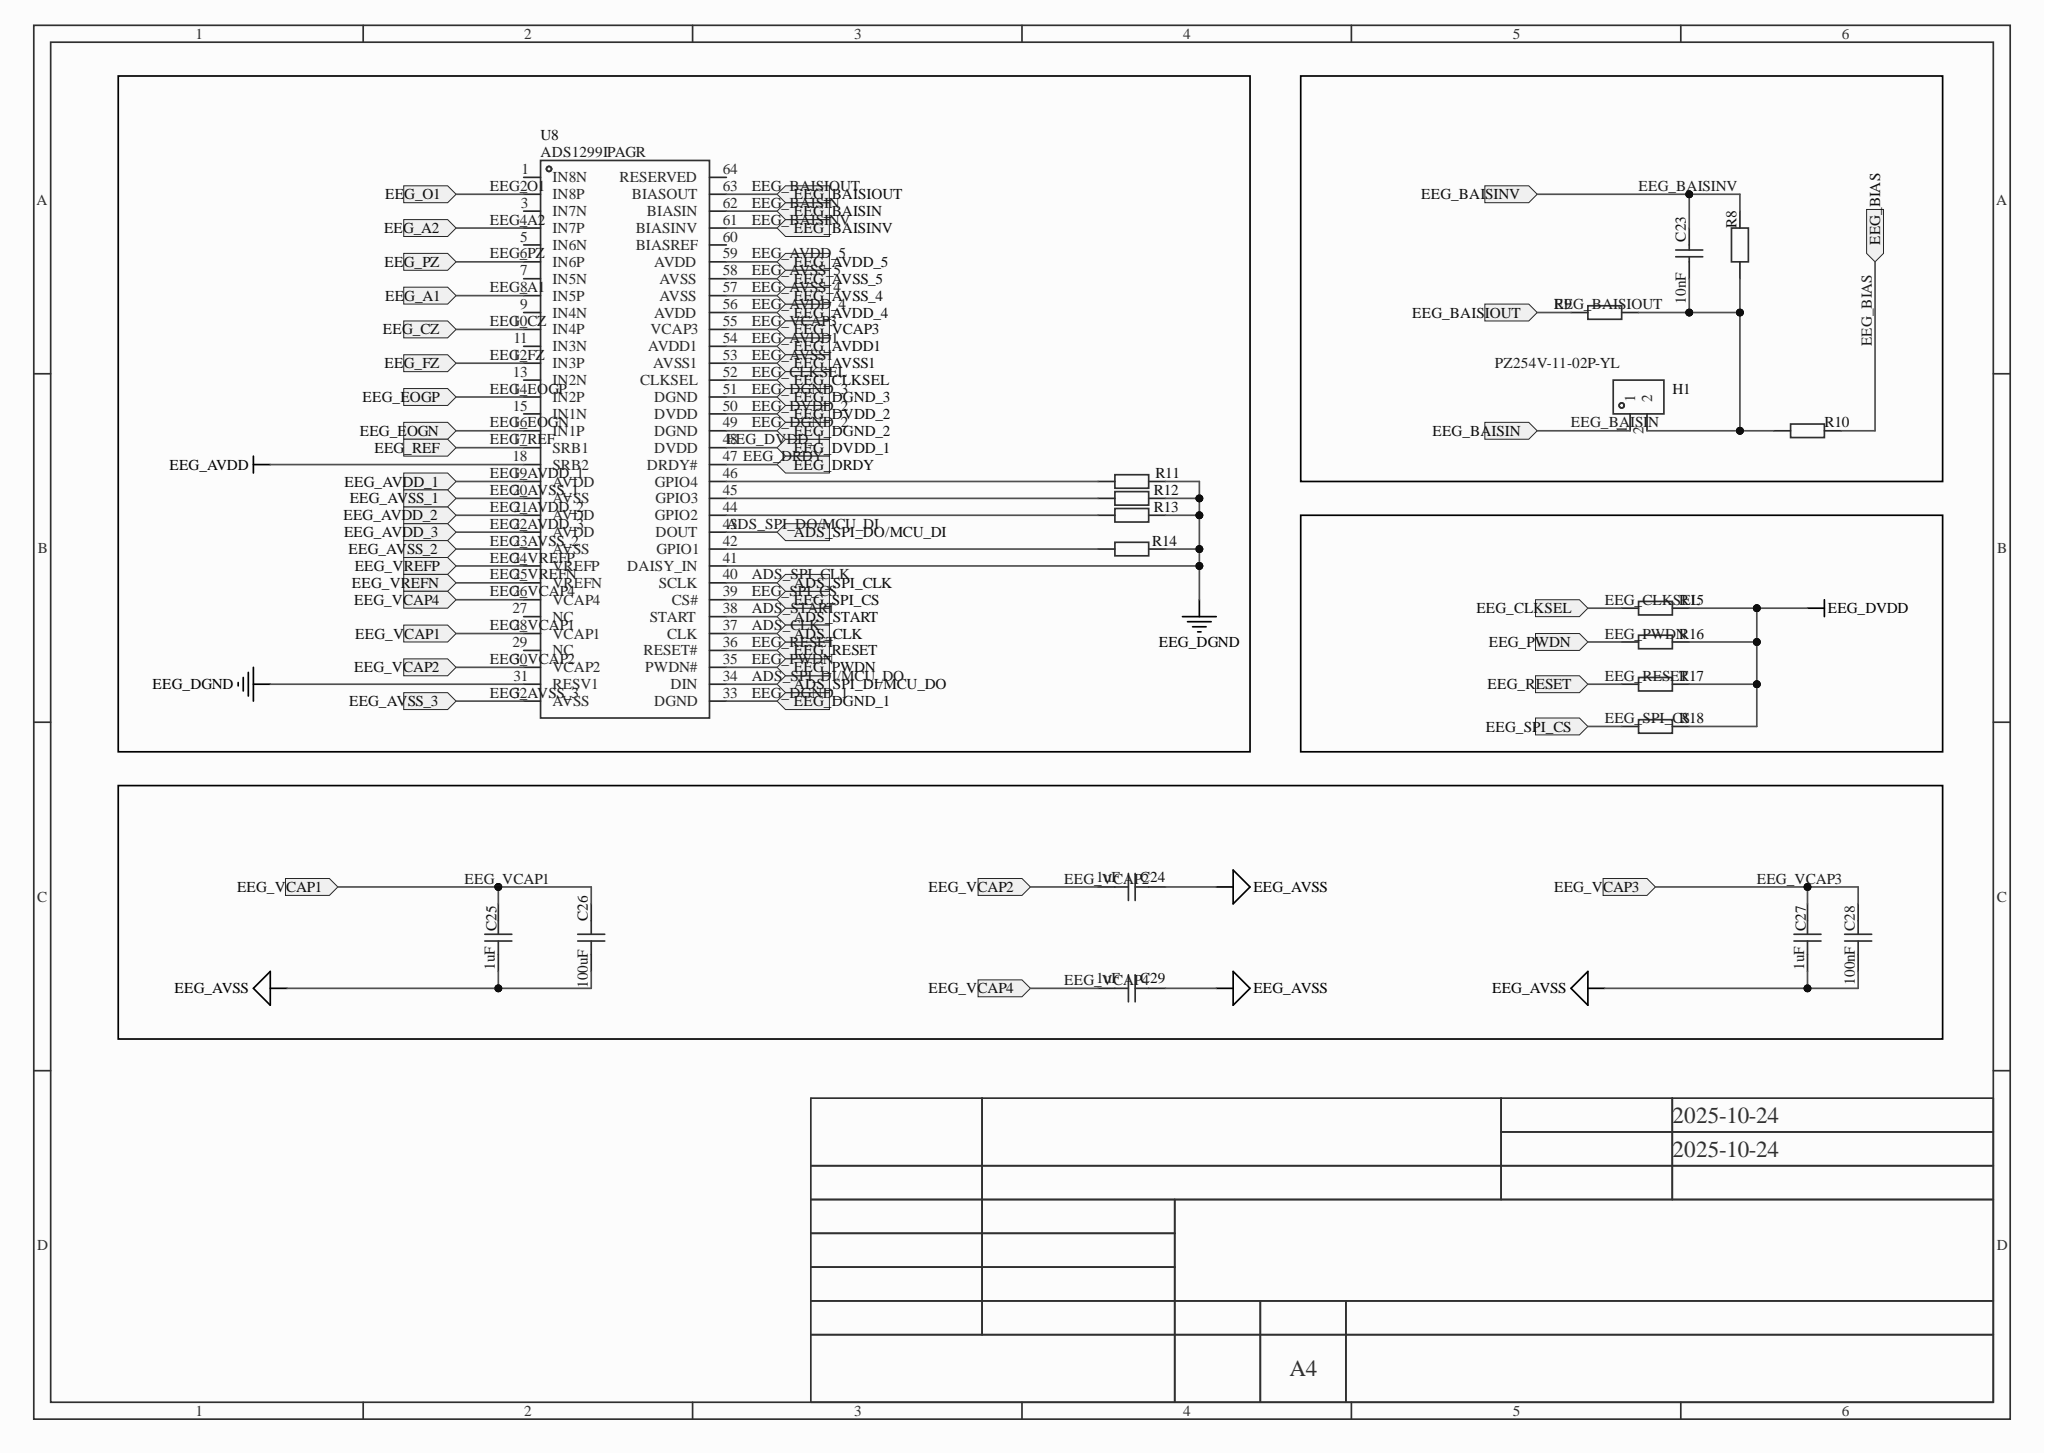Circuit board | Altium Designer | 212 parts | 123 nets | one sheet of the schematic
Parts on this sheet (reference | value | footprint):
C23 | 10nF | C0402
C24 | 1uF | C0402
C25 | 1uF | C0402
C26 | 100uF | C1206
C27 | 1uF | C0402
C28 | 100nF | C0402
C29 | 1uF | C0402
H1 | PZ254V-11-02P-YL | HDR-TH_2P-P2.54-V-M
R8 | R0402
R9 | R0402
R10 | R0402
R11 | R0402
R12 | R0402
R13 | R0402
R14 | R0402
R15 | R0402
R16 | R0402
R17 | R0402
R18 | R0402
U8 | ADS1299IPAGR | TQFP-64_L10.0-W10.0-P0.50-LS12.0-TL
Nets of these parts (net: part-pin ...):
NetR14_1: R14-1 U8-42
NetR13_1: R13-1 U8-44
NetR12_1: R12-1 U8-45
NetR11_1: R11-1 U8-46
NetC23_1: C23-1 H1-2 R8-2 R9-2 R10-1
EEG_VREFP: U8-24
EEG_VCAP4: C29-1 U8-26
EEG_VCAP3: C27-2 C28-2 U8-55
EEG_VCAP2: C24-1 U8-30
EEG_VCAP1: C25-2 C26-2 U8-28
EEG_SPI_CS: R18-1 U8-39
EEG_RESET: R17-1 U8-36
EEG_REF: U8-17
EEG_PZ: U8-6
EEG_PWDN: R16-1 U8-35
EEG_FZ: U8-12
EEG_EOGP: U8-14
EEG_EOGN: U8-16
EEG_DVDD_1: R15-2 R16-2 R17-2 R18-2 U8-48 U8-50
EEG_DRDY: U8-47
EEG_DGND_1: R11-2 R12-2 R13-2 R14-2 U8-31 U8-33 U8-41 U8-49 U8-51
EEG_CZ: U8-10
EEG_CLKSEL: R15-1 U8-52
EEG_BIAS: R10-2
EEG_BAISIOUT: R9-1 U8-63
EEG_BAISINV: C23-2 R8-1 U8-61
EEG_BAISIN: H1-1 U8-62
EEG_AVSS1: C24-2 C25-1 C26-1 C27-1 C28-1 C29-2 U8-20 U8-23 U8-25 U8-32 U8-53 U8-57 U8-58
EEG_AVDD1: U8-18 U8-19 U8-21 U8-22 U8-54 U8-56 U8-59
EEG_A1: U8-8
ADS_START: U8-38
ADS_SPI_DO/MCU_DI: U8-43
ADS_SPI_DI/MCU_DO: U8-34
ADS_SPI_CLK: U8-40
ADS_CLK: U8-37